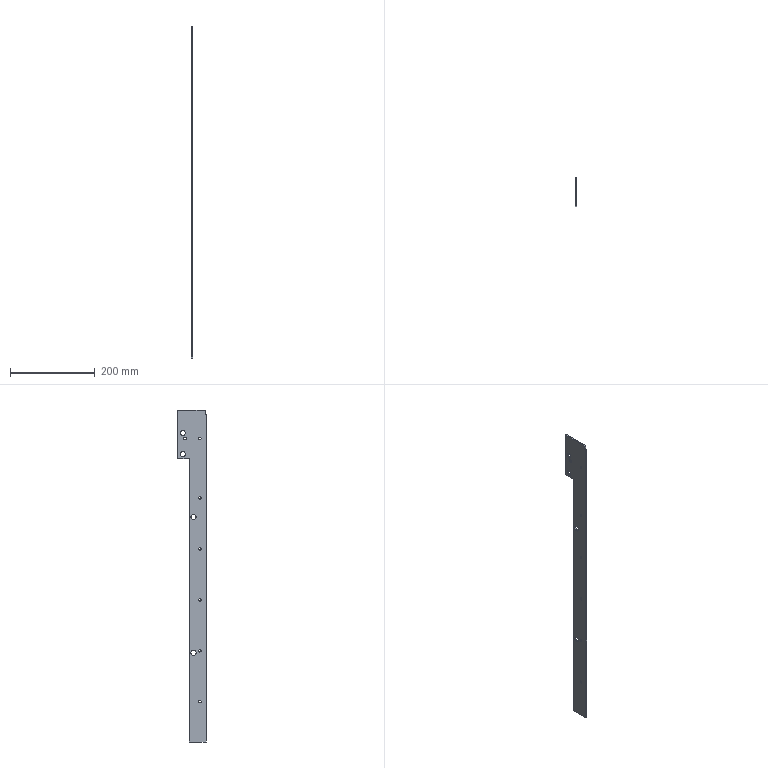Part | NX | features solid 2 | 1 solid | 32 faces | box 3 x 67 x 782.061 mm | volume 101080 mm3 | cylinder 22 | plane 10 | commonest cylinder face diameters 6 x14 12 x8
STEP:
#1=CARTESIAN_POINT('',(1112.,-680.,505.));
#2=VERTEX_POINT('',#1);
#3=CARTESIAN_POINT('',(1112.,-720.,505.));
#4=VERTEX_POINT('',#3);
#5=CARTESIAN_POINT('',(1112.,-1653.,505.));
#6=DIRECTION('',(0.,-1.,0.));
#7=VECTOR('',#6,1000.);
#8=LINE('',#5,#7);
#9=EDGE_CURVE('',#2,#4,#8,.T.);
#10=ORIENTED_EDGE('',*,*,#9,.F.);
#11=CARTESIAN_POINT('',(1115.,-680.,505.));
#12=VERTEX_POINT('',#11);
#13=CARTESIAN_POINT('',(1115.,-680.,505.));
#14=DIRECTION('',(1.,0.,0.));
#15=VECTOR('',#14,1000.);
#16=LINE('',#13,#15);
#17=EDGE_CURVE('',#2,#12,#16,.T.);
#18=ORIENTED_EDGE('',*,*,#17,.T.);
#19=CARTESIAN_POINT('',(1115.,-720.,505.));
#20=VERTEX_POINT('',#19);
#21=CARTESIAN_POINT('',(1115.,-1653.,505.));
#22=DIRECTION('',(0.,-1.,0.));
#23=VECTOR('',#22,1000.);
#24=LINE('',#21,#23);
#25=EDGE_CURVE('',#12,#20,#24,.T.);
#26=ORIENTED_EDGE('',*,*,#25,.T.);
#27=CARTESIAN_POINT('',(1115.,-720.,505.));
#28=DIRECTION('',(1.,0.,0.));
#29=VECTOR('',#28,1000.);
#30=LINE('',#27,#29);
#31=EDGE_CURVE('',#4,#20,#30,.T.);
#32=ORIENTED_EDGE('',*,*,#31,.F.);
#33=EDGE_LOOP('',(#10,#18,#26,#32));
#34=FACE_BOUND('',#33,.T.);
#35=CARTESIAN_POINT('',(1115.,-1653.,505.));
#36=DIRECTION('',(0.,0.,-1.));
#37=DIRECTION('',(0.,-1.,0.));
#38=AXIS2_PLACEMENT_3D('',#35,#36,#37);
#39=PLANE('',#38);
#40=ADVANCED_FACE('',(#34),#39,.T.);
#41=CARTESIAN_POINT('',(1112.,-717.38,1276.152));
#42=VERTEX_POINT('',#41);
#43=CARTESIAN_POINT('',(1112.,-717.38,1287.061));
#44=VERTEX_POINT('',#43);
#45=CARTESIAN_POINT('',(1112.,-717.38,0.));
#46=DIRECTION('',(0.,0.,1.));
#47=VECTOR('',#46,1000.);
#48=LINE('',#45,#47);
#49=EDGE_CURVE('',#42,#44,#48,.T.);
#50=ORIENTED_EDGE('',*,*,#49,.F.);
#51=CARTESIAN_POINT('',(1115.,-717.38,1276.152));
#52=VERTEX_POINT('',#51);
#53=CARTESIAN_POINT('',(1115.,-717.38,1276.152));
#54=DIRECTION('',(1.,0.,0.));
#55=VECTOR('',#54,1000.);
#56=LINE('',#53,#55);
#57=EDGE_CURVE('',#42,#52,#56,.T.);
#58=ORIENTED_EDGE('',*,*,#57,.T.);
#59=CARTESIAN_POINT('',(1115.,-717.38,1287.061));
#60=VERTEX_POINT('',#59);
#61=CARTESIAN_POINT('',(1115.,-717.38,0.));
#62=DIRECTION('',(0.,0.,1.));
#63=VECTOR('',#62,1000.);
#64=LINE('',#61,#63);
#65=EDGE_CURVE('',#52,#60,#64,.T.);
#66=ORIENTED_EDGE('',*,*,#65,.T.);
#67=CARTESIAN_POINT('',(1115.,-717.38,1287.061));
#68=DIRECTION('',(1.,0.,0.));
#69=VECTOR('',#68,1000.);
#70=LINE('',#67,#69);
#71=EDGE_CURVE('',#44,#60,#70,.T.);
#72=ORIENTED_EDGE('',*,*,#71,.F.);
#73=EDGE_LOOP('',(#50,#58,#66,#72));
#74=FACE_BOUND('',#73,.T.);
#75=CARTESIAN_POINT('',(1115.,-717.38,0.));
#76=DIRECTION('',(0.,-1.,0.));
#77=DIRECTION('',(-1.,0.,0.));
#78=AXIS2_PLACEMENT_3D('',#75,#76,#77);
#79=PLANE('',#78);
#80=ADVANCED_FACE('',(#74),#79,.T.);
#81=CARTESIAN_POINT('',(1112.,-720.,1276.152));
#82=VERTEX_POINT('',#81);
#83=CARTESIAN_POINT('',(1115.,-720.,1276.152));
#84=VERTEX_POINT('',#83);
#85=CARTESIAN_POINT('',(1115.,-720.,1276.152));
#86=DIRECTION('',(1.,0.,0.));
#87=VECTOR('',#86,1000.);
#88=LINE('',#85,#87);
#89=EDGE_CURVE('',#82,#84,#88,.T.);
#90=ORIENTED_EDGE('',*,*,#89,.T.);
#91=CARTESIAN_POINT('',(1115.,-1653.,1276.152));
#92=DIRECTION('',(0.,1.,0.));
#93=VECTOR('',#92,1000.);
#94=LINE('',#91,#93);
#95=EDGE_CURVE('',#84,#52,#94,.T.);
#96=ORIENTED_EDGE('',*,*,#95,.T.);
#97=ORIENTED_EDGE('',*,*,#57,.F.);
#98=CARTESIAN_POINT('',(1112.,-1653.,1276.152));
#99=DIRECTION('',(0.,1.,0.));
#100=VECTOR('',#99,1000.);
#101=LINE('',#98,#100);
#102=EDGE_CURVE('',#82,#42,#101,.T.);
#103=ORIENTED_EDGE('',*,*,#102,.F.);
#104=EDGE_LOOP('',(#90,#96,#97,#103));
#105=FACE_BOUND('',#104,.T.);
#106=CARTESIAN_POINT('',(1115.,-1653.,1276.152));
#107=DIRECTION('',(0.,0.,1.));
#108=DIRECTION('',(0.,-1.,0.));
#109=AXIS2_PLACEMENT_3D('',#106,#107,#108);
#110=PLANE('',#109);
#111=ADVANCED_FACE('',(#105),#110,.T.);
#112=CARTESIAN_POINT('',(1112.,-653.,1172.63));
#113=VERTEX_POINT('',#112);
#114=CARTESIAN_POINT('',(1115.,-653.,1172.63));
#115=VERTEX_POINT('',#114);
#116=CARTESIAN_POINT('',(1115.,-653.,1172.63));
#117=DIRECTION('',(1.,0.,0.));
#118=VECTOR('',#117,1000.);
#119=LINE('',#116,#118);
#120=EDGE_CURVE('',#113,#115,#119,.T.);
#121=ORIENTED_EDGE('',*,*,#120,.T.);
#122=CARTESIAN_POINT('',(1115.,-680.,1172.63));
#123=VERTEX_POINT('',#122);
#124=CARTESIAN_POINT('',(1115.,-1653.,1172.63));
#125=DIRECTION('',(0.,-1.,0.));
#126=VECTOR('',#125,1000.);
#127=LINE('',#124,#126);
#128=EDGE_CURVE('',#115,#123,#127,.T.);
#129=ORIENTED_EDGE('',*,*,#128,.T.);
#130=CARTESIAN_POINT('',(1112.,-680.,1172.63));
#131=VERTEX_POINT('',#130);
#132=CARTESIAN_POINT('',(1115.,-680.,1172.63));
#133=DIRECTION('',(1.,0.,0.));
#134=VECTOR('',#133,1000.);
#135=LINE('',#132,#134);
#136=EDGE_CURVE('',#131,#123,#135,.T.);
#137=ORIENTED_EDGE('',*,*,#136,.F.);
#138=CARTESIAN_POINT('',(1112.,-1653.,1172.63));
#139=DIRECTION('',(0.,1.,0.));
#140=VECTOR('',#139,1000.);
#141=LINE('',#138,#140);
#142=EDGE_CURVE('',#131,#113,#141,.T.);
#143=ORIENTED_EDGE('',*,*,#142,.T.);
#144=EDGE_LOOP('',(#121,#129,#137,#143));
#145=FACE_BOUND('',#144,.T.);
#146=CARTESIAN_POINT('',(1115.,-1653.,1172.63));
#147=DIRECTION('',(0.,0.,-1.));
#148=DIRECTION('',(0.,-1.,0.));
#149=AXIS2_PLACEMENT_3D('',#146,#147,#148);
#150=PLANE('',#149);
#151=ADVANCED_FACE('',(#145),#150,.T.);
#152=CARTESIAN_POINT('',(1115.,-680.,0.));
#153=DIRECTION('',(0.,0.,1.));
#154=VECTOR('',#153,1000.);
#155=LINE('',#152,#154);
#156=EDGE_CURVE('',#12,#123,#155,.T.);
#157=ORIENTED_EDGE('',*,*,#156,.F.);
#158=ORIENTED_EDGE('',*,*,#17,.F.);
#159=CARTESIAN_POINT('',(1112.,-680.,0.));
#160=DIRECTION('',(0.,0.,1.));
#161=VECTOR('',#160,1000.);
#162=LINE('',#159,#161);
#163=EDGE_CURVE('',#2,#131,#162,.T.);
#164=ORIENTED_EDGE('',*,*,#163,.T.);
#165=ORIENTED_EDGE('',*,*,#136,.T.);
#166=EDGE_LOOP('',(#157,#158,#164,#165));
#167=FACE_BOUND('',#166,.T.);
#168=CARTESIAN_POINT('',(1115.,-680.,0.));
#169=DIRECTION('',(0.,-1.,0.));
#170=DIRECTION('',(-1.,0.,0.));
#171=AXIS2_PLACEMENT_3D('',#168,#169,#170);
#172=PLANE('',#171);
#173=ADVANCED_FACE('',(#167),#172,.F.);
#174=CARTESIAN_POINT('',(1112.,-690.,709.));
#175=VERTEX_POINT('',#174);
#176=CARTESIAN_POINT('',(1115.,-690.,709.));
#177=VERTEX_POINT('',#176);
#178=CARTESIAN_POINT('',(-391.665,-690.,709.));
#179=DIRECTION('',(1.,0.,0.));
#180=VECTOR('',#179,1000.);
#181=LINE('',#178,#180);
#182=EDGE_CURVE('',#175,#177,#181,.T.);
#183=ORIENTED_EDGE('',*,*,#182,.F.);
#184=CARTESIAN_POINT('',(1112.,-690.,721.));
#185=VERTEX_POINT('',#184);
#186=CARTESIAN_POINT('',(1112.,-690.,715.));
#187=DIRECTION('',(-1.,0.,0.));
#188=DIRECTION('',(0.,0.,-1.));
#189=AXIS2_PLACEMENT_3D('',#186,#187,#188);
#190=CIRCLE('',#189,6.);
#191=EDGE_CURVE('',#175,#185,#190,.T.);
#192=ORIENTED_EDGE('',*,*,#191,.T.);
#193=CARTESIAN_POINT('',(1115.,-690.,721.));
#194=VERTEX_POINT('',#193);
#195=CARTESIAN_POINT('',(-391.665,-690.,721.));
#196=DIRECTION('',(1.,0.,0.));
#197=VECTOR('',#196,1000.);
#198=LINE('',#195,#197);
#199=EDGE_CURVE('',#194,#185,#198,.F.);
#200=ORIENTED_EDGE('',*,*,#199,.F.);
#201=CARTESIAN_POINT('',(1115.,-690.,715.));
#202=DIRECTION('',(1.,0.,0.));
#203=DIRECTION('',(0.,0.,-1.));
#204=AXIS2_PLACEMENT_3D('',#201,#202,#203);
#205=CIRCLE('',#204,6.);
#206=EDGE_CURVE('',#194,#177,#205,.T.);
#207=ORIENTED_EDGE('',*,*,#206,.T.);
#208=EDGE_LOOP('',(#183,#192,#200,#207));
#209=FACE_BOUND('',#208,.T.);
#210=CARTESIAN_POINT('',(-391.665,-690.,715.));
#211=DIRECTION('',(1.,0.,0.));
#212=DIRECTION('',(0.,0.,1.));
#213=AXIS2_PLACEMENT_3D('',#210,#211,#212);
#214=CYLINDRICAL_SURFACE('',#213,6.);
#215=ADVANCED_FACE('',(#209),#214,.F.);
#216=CARTESIAN_POINT('',(1115.,-690.,1029.));
#217=VERTEX_POINT('',#216);
#218=CARTESIAN_POINT('',(1112.,-690.,1029.));
#219=VERTEX_POINT('',#218);
#220=CARTESIAN_POINT('',(-391.665,-690.,1029.));
#221=DIRECTION('',(1.,0.,0.));
#222=VECTOR('',#221,1000.);
#223=LINE('',#220,#222);
#224=EDGE_CURVE('',#217,#219,#223,.F.);
#225=ORIENTED_EDGE('',*,*,#224,.T.);
#226=CARTESIAN_POINT('',(1112.,-690.,1041.));
#227=VERTEX_POINT('',#226);
#228=CARTESIAN_POINT('',(1112.,-690.,1035.));
#229=DIRECTION('',(-1.,0.,0.));
#230=DIRECTION('',(0.,0.,-1.));
#231=AXIS2_PLACEMENT_3D('',#228,#229,#230);
#232=CIRCLE('',#231,6.);
#233=EDGE_CURVE('',#219,#227,#232,.T.);
#234=ORIENTED_EDGE('',*,*,#233,.T.);
#235=CARTESIAN_POINT('',(1115.,-690.,1041.));
#236=VERTEX_POINT('',#235);
#237=CARTESIAN_POINT('',(-391.665,-690.,1041.));
#238=DIRECTION('',(1.,0.,0.));
#239=VECTOR('',#238,1000.);
#240=LINE('',#237,#239);
#241=EDGE_CURVE('',#227,#236,#240,.T.);
#242=ORIENTED_EDGE('',*,*,#241,.T.);
#243=CARTESIAN_POINT('',(1115.,-690.,1035.));
#244=DIRECTION('',(1.,0.,0.));
#245=DIRECTION('',(0.,0.,-1.));
#246=AXIS2_PLACEMENT_3D('',#243,#244,#245);
#247=CIRCLE('',#246,6.);
#248=EDGE_CURVE('',#236,#217,#247,.T.);
#249=ORIENTED_EDGE('',*,*,#248,.T.);
#250=EDGE_LOOP('',(#225,#234,#242,#249));
#251=FACE_BOUND('',#250,.T.);
#252=CARTESIAN_POINT('',(-391.665,-690.,1035.));
#253=DIRECTION('',(1.,0.,0.));
#254=DIRECTION('',(0.,0.,1.));
#255=AXIS2_PLACEMENT_3D('',#252,#253,#254);
#256=CYLINDRICAL_SURFACE('',#255,6.);
#257=ADVANCED_FACE('',(#251),#256,.F.);
#258=CARTESIAN_POINT('',(1112.,-665.,1177.061));
#259=VERTEX_POINT('',#258);
#260=CARTESIAN_POINT('',(1115.,-665.,1177.061));
#261=VERTEX_POINT('',#260);
#262=CARTESIAN_POINT('',(-391.665,-665.,1177.061));
#263=DIRECTION('',(1.,0.,0.));
#264=VECTOR('',#263,1000.);
#265=LINE('',#262,#264);
#266=EDGE_CURVE('',#259,#261,#265,.T.);
#267=ORIENTED_EDGE('',*,*,#266,.F.);
#268=CARTESIAN_POINT('',(1112.,-665.,1189.061));
#269=VERTEX_POINT('',#268);
#270=CARTESIAN_POINT('',(1112.,-665.,1183.061));
#271=DIRECTION('',(-1.,0.,0.));
#272=DIRECTION('',(0.,0.,-1.));
#273=AXIS2_PLACEMENT_3D('',#270,#271,#272);
#274=CIRCLE('',#273,6.);
#275=EDGE_CURVE('',#259,#269,#274,.T.);
#276=ORIENTED_EDGE('',*,*,#275,.T.);
#277=CARTESIAN_POINT('',(1115.,-665.,1189.061));
#278=VERTEX_POINT('',#277);
#279=CARTESIAN_POINT('',(-391.665,-665.,1189.061));
#280=DIRECTION('',(1.,0.,0.));
#281=VECTOR('',#280,1000.);
#282=LINE('',#279,#281);
#283=EDGE_CURVE('',#278,#269,#282,.F.);
#284=ORIENTED_EDGE('',*,*,#283,.F.);
#285=CARTESIAN_POINT('',(1115.,-665.,1183.061));
#286=DIRECTION('',(1.,0.,0.));
#287=DIRECTION('',(0.,0.,-1.));
#288=AXIS2_PLACEMENT_3D('',#285,#286,#287);
#289=CIRCLE('',#288,6.);
#290=EDGE_CURVE('',#278,#261,#289,.T.);
#291=ORIENTED_EDGE('',*,*,#290,.T.);
#292=EDGE_LOOP('',(#267,#276,#284,#291));
#293=FACE_BOUND('',#292,.T.);
#294=CARTESIAN_POINT('',(-391.665,-665.,1183.061));
#295=DIRECTION('',(1.,0.,0.));
#296=DIRECTION('',(0.,0.,1.));
#297=AXIS2_PLACEMENT_3D('',#294,#295,#296);
#298=CYLINDRICAL_SURFACE('',#297,6.);
#299=ADVANCED_FACE('',(#293),#298,.F.);
#300=CARTESIAN_POINT('',(1115.,-665.,1227.061));
#301=VERTEX_POINT('',#300);
#302=CARTESIAN_POINT('',(1112.,-665.,1227.061));
#303=VERTEX_POINT('',#302);
#304=CARTESIAN_POINT('',(-391.665,-665.,1227.061));
#305=DIRECTION('',(1.,0.,0.));
#306=VECTOR('',#305,1000.);
#307=LINE('',#304,#306);
#308=EDGE_CURVE('',#301,#303,#307,.F.);
#309=ORIENTED_EDGE('',*,*,#308,.T.);
#310=CARTESIAN_POINT('',(1112.,-665.,1239.061));
#311=VERTEX_POINT('',#310);
#312=CARTESIAN_POINT('',(1112.,-665.,1233.061));
#313=DIRECTION('',(-1.,0.,0.));
#314=DIRECTION('',(0.,0.,-1.));
#315=AXIS2_PLACEMENT_3D('',#312,#313,#314);
#316=CIRCLE('',#315,6.);
#317=EDGE_CURVE('',#303,#311,#316,.T.);
#318=ORIENTED_EDGE('',*,*,#317,.T.);
#319=CARTESIAN_POINT('',(1115.,-665.,1239.061));
#320=VERTEX_POINT('',#319);
#321=CARTESIAN_POINT('',(-391.665,-665.,1239.061));
#322=DIRECTION('',(1.,0.,0.));
#323=VECTOR('',#322,1000.);
#324=LINE('',#321,#323);
#325=EDGE_CURVE('',#311,#320,#324,.T.);
#326=ORIENTED_EDGE('',*,*,#325,.T.);
#327=CARTESIAN_POINT('',(1115.,-665.,1233.061));
#328=DIRECTION('',(1.,0.,0.));
#329=DIRECTION('',(0.,0.,-1.));
#330=AXIS2_PLACEMENT_3D('',#327,#328,#329);
#331=CIRCLE('',#330,6.);
#332=EDGE_CURVE('',#320,#301,#331,.T.);
#333=ORIENTED_EDGE('',*,*,#332,.T.);
#334=EDGE_LOOP('',(#309,#318,#326,#333));
#335=FACE_BOUND('',#334,.T.);
#336=CARTESIAN_POINT('',(-391.665,-665.,1233.061));
#337=DIRECTION('',(1.,0.,0.));
#338=DIRECTION('',(0.,0.,1.));
#339=AXIS2_PLACEMENT_3D('',#336,#337,#338);
#340=CYLINDRICAL_SURFACE('',#339,6.);
#341=ADVANCED_FACE('',(#335),#340,.F.);
#342=CARTESIAN_POINT('',(1112.,-705.,1217.));
#343=VERTEX_POINT('',#342);
#344=CARTESIAN_POINT('',(1115.,-705.,1217.));
#345=VERTEX_POINT('',#344);
#346=CARTESIAN_POINT('',(-391.665,-705.,1217.));
#347=DIRECTION('',(1.,0.,0.));
#348=VECTOR('',#347,1000.);
#349=LINE('',#346,#348);
#350=EDGE_CURVE('',#343,#345,#349,.T.);
#351=ORIENTED_EDGE('',*,*,#350,.F.);
#352=CARTESIAN_POINT('',(1112.,-705.,1223.));
#353=VERTEX_POINT('',#352);
#354=CARTESIAN_POINT('',(1112.,-705.,1220.));
#355=DIRECTION('',(1.,0.,0.));
#356=DIRECTION('',(0.,0.,-1.));
#357=AXIS2_PLACEMENT_3D('',#354,#355,#356);
#358=CIRCLE('',#357,3.);
#359=EDGE_CURVE('',#353,#343,#358,.T.);
#360=ORIENTED_EDGE('',*,*,#359,.F.);
#361=CARTESIAN_POINT('',(1115.,-705.,1223.));
#362=VERTEX_POINT('',#361);
#363=CARTESIAN_POINT('',(-391.665,-705.,1223.));
#364=DIRECTION('',(1.,0.,0.));
#365=VECTOR('',#364,1000.);
#366=LINE('',#363,#365);
#367=EDGE_CURVE('',#362,#353,#366,.F.);
#368=ORIENTED_EDGE('',*,*,#367,.F.);
#369=CARTESIAN_POINT('',(1115.,-705.,1220.));
#370=DIRECTION('',(-1.,0.,0.));
#371=DIRECTION('',(0.,1.,0.));
#372=AXIS2_PLACEMENT_3D('',#369,#370,#371);
#373=CIRCLE('',#372,3.);
#374=EDGE_CURVE('',#345,#362,#373,.T.);
#375=ORIENTED_EDGE('',*,*,#374,.F.);
#376=EDGE_LOOP('',(#351,#360,#368,#375));
#377=FACE_BOUND('',#376,.T.);
#378=CARTESIAN_POINT('',(-391.665,-705.,1220.));
#379=DIRECTION('',(1.,0.,0.));
#380=DIRECTION('',(0.,0.,1.));
#381=AXIS2_PLACEMENT_3D('',#378,#379,#380);
#382=CYLINDRICAL_SURFACE('',#381,3.);
#383=ADVANCED_FACE('',(#377),#382,.F.);
#384=CARTESIAN_POINT('',(1112.,-670.,1217.));
#385=VERTEX_POINT('',#384);
#386=CARTESIAN_POINT('',(1115.,-670.,1217.));
#387=VERTEX_POINT('',#386);
#388=CARTESIAN_POINT('',(-391.665,-670.,1217.));
#389=DIRECTION('',(1.,0.,0.));
#390=VECTOR('',#389,1000.);
#391=LINE('',#388,#390);
#392=EDGE_CURVE('',#385,#387,#391,.T.);
#393=ORIENTED_EDGE('',*,*,#392,.F.);
#394=CARTESIAN_POINT('',(1112.,-670.,1223.));
#395=VERTEX_POINT('',#394);
#396=CARTESIAN_POINT('',(1112.,-670.,1220.));
#397=DIRECTION('',(1.,0.,0.));
#398=DIRECTION('',(0.,0.,-1.));
#399=AXIS2_PLACEMENT_3D('',#396,#397,#398);
#400=CIRCLE('',#399,3.);
#401=EDGE_CURVE('',#395,#385,#400,.T.);
#402=ORIENTED_EDGE('',*,*,#401,.F.);
#403=CARTESIAN_POINT('',(1115.,-670.,1223.));
#404=VERTEX_POINT('',#403);
#405=CARTESIAN_POINT('',(-391.665,-670.,1223.));
#406=DIRECTION('',(1.,0.,0.));
#407=VECTOR('',#406,1000.);
#408=LINE('',#405,#407);
#409=EDGE_CURVE('',#404,#395,#408,.F.);
#410=ORIENTED_EDGE('',*,*,#409,.F.);
#411=CARTESIAN_POINT('',(1115.,-670.,1220.));
#412=DIRECTION('',(-1.,0.,0.));
#413=DIRECTION('',(0.,1.,0.));
#414=AXIS2_PLACEMENT_3D('',#411,#412,#413);
#415=CIRCLE('',#414,3.);
#416=EDGE_CURVE('',#387,#404,#415,.T.);
#417=ORIENTED_EDGE('',*,*,#416,.F.);
#418=EDGE_LOOP('',(#393,#402,#410,#417));
#419=FACE_BOUND('',#418,.T.);
#420=CARTESIAN_POINT('',(-391.665,-670.,1220.));
#421=DIRECTION('',(1.,0.,0.));
#422=DIRECTION('',(0.,0.,1.));
#423=AXIS2_PLACEMENT_3D('',#420,#421,#422);
#424=CYLINDRICAL_SURFACE('',#423,3.);
#425=ADVANCED_FACE('',(#419),#424,.F.);
#426=CARTESIAN_POINT('',(1115.,-705.,1077.));
#427=VERTEX_POINT('',#426);
#428=CARTESIAN_POINT('',(1112.,-705.,1077.));
#429=VERTEX_POINT('',#428);
#430=CARTESIAN_POINT('',(-391.665,-705.,1077.));
#431=DIRECTION('',(1.,0.,0.));
#432=VECTOR('',#431,1000.);
#433=LINE('',#430,#432);
#434=EDGE_CURVE('',#427,#429,#433,.F.);
#435=ORIENTED_EDGE('',*,*,#434,.T.);
#436=CARTESIAN_POINT('',(1112.,-705.,1083.));
#437=VERTEX_POINT('',#436);
#438=CARTESIAN_POINT('',(1112.,-705.,1080.));
#439=DIRECTION('',(1.,0.,0.));
#440=DIRECTION('',(0.,0.,-1.));
#441=AXIS2_PLACEMENT_3D('',#438,#439,#440);
#442=CIRCLE('',#441,3.);
#443=EDGE_CURVE('',#437,#429,#442,.T.);
#444=ORIENTED_EDGE('',*,*,#443,.F.);
#445=CARTESIAN_POINT('',(1115.,-705.,1083.));
#446=VERTEX_POINT('',#445);
#447=CARTESIAN_POINT('',(-391.665,-705.,1083.));
#448=DIRECTION('',(1.,0.,0.));
#449=VECTOR('',#448,1000.);
#450=LINE('',#447,#449);
#451=EDGE_CURVE('',#437,#446,#450,.T.);
#452=ORIENTED_EDGE('',*,*,#451,.T.);
#453=CARTESIAN_POINT('',(1115.,-705.,1080.));
#454=DIRECTION('',(-1.,0.,0.));
#455=DIRECTION('',(0.,1.,0.));
#456=AXIS2_PLACEMENT_3D('',#453,#454,#455);
#457=CIRCLE('',#456,3.);
#458=EDGE_CURVE('',#427,#446,#457,.T.);
#459=ORIENTED_EDGE('',*,*,#458,.F.);
#460=EDGE_LOOP('',(#435,#444,#452,#459));
#461=FACE_BOUND('',#460,.T.);
#462=CARTESIAN_POINT('',(-391.665,-705.,1080.));
#463=DIRECTION('',(1.,0.,0.));
#464=DIRECTION('',(0.,0.,1.));
#465=AXIS2_PLACEMENT_3D('',#462,#463,#464);
#466=CYLINDRICAL_SURFACE('',#465,3.);
#467=ADVANCED_FACE('',(#461),#466,.F.);
#468=CARTESIAN_POINT('',(1112.,-705.,957.));
#469=VERTEX_POINT('',#468);
#470=CARTESIAN_POINT('',(1115.,-705.,957.));
#471=VERTEX_POINT('',#470);
#472=CARTESIAN_POINT('',(-391.665,-705.,957.));
#473=DIRECTION('',(1.,0.,0.));
#474=VECTOR('',#473,1000.);
#475=LINE('',#472,#474);
#476=EDGE_CURVE('',#469,#471,#475,.T.);
#477=ORIENTED_EDGE('',*,*,#476,.F.);
#478=CARTESIAN_POINT('',(1112.,-705.,963.));
#479=VERTEX_POINT('',#478);
#480=CARTESIAN_POINT('',(1112.,-705.,960.));
#481=DIRECTION('',(1.,0.,0.));
#482=DIRECTION('',(0.,0.,-1.));
#483=AXIS2_PLACEMENT_3D('',#480,#481,#482);
#484=CIRCLE('',#483,3.);
#485=EDGE_CURVE('',#479,#469,#484,.T.);
#486=ORIENTED_EDGE('',*,*,#485,.F.);
#487=CARTESIAN_POINT('',(1115.,-705.,963.));
#488=VERTEX_POINT('',#487);
#489=CARTESIAN_POINT('',(-391.665,-705.,963.));
#490=DIRECTION('',(1.,0.,0.));
#491=VECTOR('',#490,1000.);
#492=LINE('',#489,#491);
#493=EDGE_CURVE('',#488,#479,#492,.F.);
#494=ORIENTED_EDGE('',*,*,#493,.F.);
#495=CARTESIAN_POINT('',(1115.,-705.,960.));
#496=DIRECTION('',(-1.,0.,0.));
#497=DIRECTION('',(0.,1.,0.));
#498=AXIS2_PLACEMENT_3D('',#495,#496,#497);
#499=CIRCLE('',#498,3.);
#500=EDGE_CURVE('',#471,#488,#499,.T.);
#501=ORIENTED_EDGE('',*,*,#500,.F.);
#502=EDGE_LOOP('',(#477,#486,#494,#501));
#503=FACE_BOUND('',#502,.T.);
#504=CARTESIAN_POINT('',(-391.665,-705.,960.));
#505=DIRECTION('',(1.,0.,0.));
#506=DIRECTION('',(0.,0.,1.));
#507=AXIS2_PLACEMENT_3D('',#504,#505,#506);
#508=CYLINDRICAL_SURFACE('',#507,3.);
#509=ADVANCED_FACE('',(#503),#508,.F.);
#510=CARTESIAN_POINT('',(1115.,-705.,837.));
#511=VERTEX_POINT('',#510);
#512=CARTESIAN_POINT('',(1112.,-705.,837.));
#513=VERTEX_POINT('',#512);
#514=CARTESIAN_POINT('',(-391.665,-705.,837.));
#515=DIRECTION('',(1.,0.,0.));
#516=VECTOR('',#515,1000.);
#517=LINE('',#514,#516);
#518=EDGE_CURVE('',#511,#513,#517,.F.);
#519=ORIENTED_EDGE('',*,*,#518,.T.);
#520=CARTESIAN_POINT('',(1112.,-705.,843.));
#521=VERTEX_POINT('',#520);
#522=CARTESIAN_POINT('',(1112.,-705.,840.));
#523=DIRECTION('',(1.,0.,0.));
#524=DIRECTION('',(0.,0.,-1.));
#525=AXIS2_PLACEMENT_3D('',#522,#523,#524);
#526=CIRCLE('',#525,3.);
#527=EDGE_CURVE('',#521,#513,#526,.T.);
#528=ORIENTED_EDGE('',*,*,#527,.F.);
#529=CARTESIAN_POINT('',(1115.,-705.,843.));
#530=VERTEX_POINT('',#529);
#531=CARTESIAN_POINT('',(-391.665,-705.,843.));
#532=DIRECTION('',(1.,0.,0.));
#533=VECTOR('',#532,1000.);
#534=LINE('',#531,#533);
#535=EDGE_CURVE('',#521,#530,#534,.T.);
#536=ORIENTED_EDGE('',*,*,#535,.T.);
#537=CARTESIAN_POINT('',(1115.,-705.,840.));
#538=DIRECTION('',(-1.,0.,0.));
#539=DIRECTION('',(0.,1.,0.));
#540=AXIS2_PLACEMENT_3D('',#537,#538,#539);
#541=CIRCLE('',#540,3.);
#542=EDGE_CURVE('',#511,#530,#541,.T.);
#543=ORIENTED_EDGE('',*,*,#542,.F.);
#544=EDGE_LOOP('',(#519,#528,#536,#543));
#545=FACE_BOUND('',#544,.T.);
#546=CARTESIAN_POINT('',(-391.665,-705.,840.));
#547=DIRECTION('',(1.,0.,0.));
#548=DIRECTION('',(0.,0.,1.));
#549=AXIS2_PLACEMENT_3D('',#546,#547,#548);
#550=CYLINDRICAL_SURFACE('',#549,3.);
#551=ADVANCED_FACE('',(#545),#550,.F.);
#552=CARTESIAN_POINT('',(1112.,-705.,717.));
#553=VERTEX_POINT('',#552);
#554=CARTESIAN_POINT('',(1115.,-705.,717.));
#555=VERTEX_POINT('',#554);
#556=CARTESIAN_POINT('',(-391.665,-705.,717.));
#557=DIRECTION('',(1.,0.,0.));
#558=VECTOR('',#557,1000.);
#559=LINE('',#556,#558);
#560=EDGE_CURVE('',#553,#555,#559,.T.);
#561=ORIENTED_EDGE('',*,*,#560,.F.);
#562=CARTESIAN_POINT('',(1112.,-705.,723.));
#563=VERTEX_POINT('',#562);
#564=CARTESIAN_POINT('',(1112.,-705.,720.));
#565=DIRECTION('',(1.,0.,0.));
#566=DIRECTION('',(0.,0.,-1.));
#567=AXIS2_PLACEMENT_3D('',#564,#565,#566);
#568=CIRCLE('',#567,3.);
#569=EDGE_CURVE('',#563,#553,#568,.T.);
#570=ORIENTED_EDGE('',*,*,#569,.F.);
#571=CARTESIAN_POINT('',(1115.,-705.,723.));
#572=VERTEX_POINT('',#571);
#573=CARTESIAN_POINT('',(-391.665,-705.,723.));
#574=DIRECTION('',(1.,0.,0.));
#575=VECTOR('',#574,1000.);
#576=LINE('',#573,#575);
#577=EDGE_CURVE('',#572,#563,#576,.F.);
#578=ORIENTED_EDGE('',*,*,#577,.F.);
#579=CARTESIAN_POINT('',(1115.,-705.,720.));
#580=DIRECTION('',(-1.,0.,0.));
#581=DIRECTION('',(0.,1.,0.));
#582=AXIS2_PLACEMENT_3D('',#579,#580,#581);
#583=CIRCLE('',#582,3.);
#584=EDGE_CURVE('',#555,#572,#583,.T.);
#585=ORIENTED_EDGE('',*,*,#584,.F.);
#586=EDGE_LOOP('',(#561,#570,#578,#585));
#587=FACE_BOUND('',#586,.T.);
#588=CARTESIAN_POINT('',(-391.665,-705.,720.));
#589=DIRECTION('',(1.,0.,0.));
#590=DIRECTION('',(0.,0.,1.));
#591=AXIS2_PLACEMENT_3D('',#588,#589,#590);
#592=CYLINDRICAL_SURFACE('',#591,3.);
#593=ADVANCED_FACE('',(#587),#592,.F.);
#594=CARTESIAN_POINT('',(1112.,-705.,597.));
#595=VERTEX_POINT('',#594);
#596=CARTESIAN_POINT('',(1115.,-705.,597.));
#597=VERTEX_POINT('',#596);
#598=CARTESIAN_POINT('',(-391.665,-705.,597.));
#599=DIRECTION('',(1.,0.,0.));
#600=VECTOR('',#599,1000.);
#601=LINE('',#598,#600);
#602=EDGE_CURVE('',#595,#597,#601,.T.);
#603=ORIENTED_EDGE('',*,*,#602,.F.);
#604=CARTESIAN_POINT('',(1112.,-705.,603.));
#605=VERTEX_POINT('',#604);
#606=CARTESIAN_POINT('',(1112.,-705.,600.));
#607=DIRECTION('',(1.,0.,0.));
#608=DIRECTION('',(0.,0.,-1.));
#609=AXIS2_PLACEMENT_3D('',#606,#607,#608);
#610=CIRCLE('',#609,3.);
#611=EDGE_CURVE('',#605,#595,#610,.T.);
#612=ORIENTED_EDGE('',*,*,#611,.F.);
#613=CARTESIAN_POINT('',(1115.,-705.,603.));
#614=VERTEX_POINT('',#613);
#615=CARTESIAN_POINT('',(-391.665,-705.,603.));
#616=DIRECTION('',(1.,0.,0.));
#617=VECTOR('',#616,1000.);
#618=LINE('',#615,#617);
#619=EDGE_CURVE('',#614,#605,#618,.F.);
#620=ORIENTED_EDGE('',*,*,#619,.F.);
#621=CARTESIAN_POINT('',(1115.,-705.,600.));
#622=DIRECTION('',(-1.,0.,0.));
#623=DIRECTION('',(0.,1.,0.));
#624=AXIS2_PLACEMENT_3D('',#621,#622,#623);
#625=CIRCLE('',#624,3.);
#626=EDGE_CURVE('',#597,#614,#625,.T.);
#627=ORIENTED_EDGE('',*,*,#626,.F.);
#628=EDGE_LOOP('',(#603,#612,#620,#627));
#629=FACE_BOUND('',#628,.T.);
#630=CARTESIAN_POINT('',(-391.665,-705.,600.));
#631=DIRECTION('',(1.,0.,0.));
#632=DIRECTION('',(0.,0.,1.));
#633=AXIS2_PLACEMENT_3D('',#630,#631,#632);
#634=CYLINDRICAL_SURFACE('',#633,3.);
#635=ADVANCED_FACE('',(#629),#634,.F.);
#636=CARTESIAN_POINT('',(1115.,-705.,600.));
#637=DIRECTION('',(-1.,0.,0.));
#638=DIRECTION('',(0.,1.,0.));
#639=AXIS2_PLACEMENT_3D('',#636,#637,#638);
#640=CIRCLE('',#639,3.);
#641=EDGE_CURVE('',#614,#597,#640,.T.);
#642=ORIENTED_EDGE('',*,*,#641,.T.);
#643=ORIENTED_EDGE('',*,*,#626,.T.);
#644=EDGE_LOOP('',(#642,#643));
#645=FACE_BOUND('',#644,.T.);
#646=CARTESIAN_POINT('',(1115.,-705.,720.));
#647=DIRECTION('',(-1.,0.,0.));
#648=DIRECTION('',(0.,1.,0.));
#649=AXIS2_PLACEMENT_3D('',#646,#647,#648);
#650=CIRCLE('',#649,3.);
#651=EDGE_CURVE('',#572,#555,#650,.T.);
#652=ORIENTED_EDGE('',*,*,#651,.T.);
#653=ORIENTED_EDGE('',*,*,#584,.T.);
#654=EDGE_LOOP('',(#652,#653));
#655=FACE_BOUND('',#654,.T.);
#656=CARTESIAN_POINT('',(1115.,-705.,840.));
#657=DIRECTION('',(-1.,0.,0.));
#658=DIRECTION('',(0.,1.,0.));
#659=AXIS2_PLACEMENT_3D('',#656,#657,#658);
#660=CIRCLE('',#659,3.);
#661=EDGE_CURVE('',#530,#511,#660,.T.);
#662=ORIENTED_EDGE('',*,*,#661,.T.);
#663=ORIENTED_EDGE('',*,*,#542,.T.);
#664=EDGE_LOOP('',(#662,#663));
#665=FACE_BOUND('',#664,.T.);
#666=CARTESIAN_POINT('',(1115.,-705.,960.));
#667=DIRECTION('',(-1.,0.,0.));
#668=DIRECTION('',(0.,1.,0.));
#669=AXIS2_PLACEMENT_3D('',#666,#667,#668);
#670=CIRCLE('',#669,3.);
#671=EDGE_CURVE('',#488,#471,#670,.T.);
#672=ORIENTED_EDGE('',*,*,#671,.T.);
#673=ORIENTED_EDGE('',*,*,#500,.T.);
#674=EDGE_LOOP('',(#672,#673));
#675=FACE_BOUND('',#674,.T.);
#676=CARTESIAN_POINT('',(1115.,-705.,1080.));
#677=DIRECTION('',(-1.,0.,0.));
#678=DIRECTION('',(0.,1.,0.));
#679=AXIS2_PLACEMENT_3D('',#676,#677,#678);
#680=CIRCLE('',#679,3.);
#681=EDGE_CURVE('',#446,#427,#680,.T.);
#682=ORIENTED_EDGE('',*,*,#681,.T.);
#683=ORIENTED_EDGE('',*,*,#458,.T.);
#684=EDGE_LOOP('',(#682,#683));
#685=FACE_BOUND('',#684,.T.);
#686=CARTESIAN_POINT('',(1115.,-670.,1220.));
#687=DIRECTION('',(-1.,0.,0.));
#688=DIRECTION('',(0.,1.,0.));
#689=AXIS2_PLACEMENT_3D('',#686,#687,#688);
#690=CIRCLE('',#689,3.);
#691=EDGE_CURVE('',#404,#387,#690,.T.);
#692=ORIENTED_EDGE('',*,*,#691,.T.);
#693=ORIENTED_EDGE('',*,*,#416,.T.);
#694=EDGE_LOOP('',(#692,#693));
#695=FACE_BOUND('',#694,.T.);
#696=CARTESIAN_POINT('',(1115.,-705.,1220.));
#697=DIRECTION('',(-1.,0.,0.));
#698=DIRECTION('',(0.,1.,0.));
#699=AXIS2_PLACEMENT_3D('',#696,#697,#698);
#700=CIRCLE('',#699,3.);
#701=EDGE_CURVE('',#362,#345,#700,.T.);
#702=ORIENTED_EDGE('',*,*,#701,.T.);
#703=ORIENTED_EDGE('',*,*,#374,.T.);
#704=EDGE_LOOP('',(#702,#703));
#705=FACE_BOUND('',#704,.T.);
#706=ORIENTED_EDGE('',*,*,#332,.F.);
#707=CARTESIAN_POINT('',(1115.,-665.,1233.061));
#708=DIRECTION('',(1.,0.,0.));
#709=DIRECTION('',(0.,0.,-1.));
#710=AXIS2_PLACEMENT_3D('',#707,#708,#709);
#711=CIRCLE('',#710,6.);
#712=EDGE_CURVE('',#301,#320,#711,.T.);
#713=ORIENTED_EDGE('',*,*,#712,.F.);
#714=EDGE_LOOP('',(#706,#713));
#715=FACE_BOUND('',#714,.T.);
#716=ORIENTED_EDGE('',*,*,#290,.F.);
#717=CARTESIAN_POINT('',(1115.,-665.,1183.061));
#718=DIRECTION('',(1.,0.,0.));
#719=DIRECTION('',(0.,0.,-1.));
#720=AXIS2_PLACEMENT_3D('',#717,#718,#719);
#721=CIRCLE('',#720,6.);
#722=EDGE_CURVE('',#261,#278,#721,.T.);
#723=ORIENTED_EDGE('',*,*,#722,.F.);
#724=EDGE_LOOP('',(#716,#723));
#725=FACE_BOUND('',#724,.T.);
#726=ORIENTED_EDGE('',*,*,#248,.F.);
#727=CARTESIAN_POINT('',(1115.,-690.,1035.));
#728=DIRECTION('',(1.,0.,0.));
#729=DIRECTION('',(0.,0.,-1.));
#730=AXIS2_PLACEMENT_3D('',#727,#728,#729);
#731=CIRCLE('',#730,6.);
#732=EDGE_CURVE('',#217,#236,#731,.T.);
#733=ORIENTED_EDGE('',*,*,#732,.F.);
#734=EDGE_LOOP('',(#726,#733));
#735=FACE_BOUND('',#734,.T.);
#736=ORIENTED_EDGE('',*,*,#206,.F.);
#737=CARTESIAN_POINT('',(1115.,-690.,715.));
#738=DIRECTION('',(1.,0.,0.));
#739=DIRECTION('',(0.,0.,-1.));
#740=AXIS2_PLACEMENT_3D('',#737,#738,#739);
#741=CIRCLE('',#740,6.);
#742=EDGE_CURVE('',#177,#194,#741,.T.);
#743=ORIENTED_EDGE('',*,*,#742,.F.);
#744=EDGE_LOOP('',(#736,#743));
#745=FACE_BOUND('',#744,.T.);
#746=CARTESIAN_POINT('',(1115.,-720.,1287.061));
#747=DIRECTION('',(0.,0.,-1.));
#748=VECTOR('',#747,1000.);
#749=LINE('',#746,#748);
#750=EDGE_CURVE('',#84,#20,#749,.T.);
#751=ORIENTED_EDGE('',*,*,#750,.T.);
#752=ORIENTED_EDGE('',*,*,#25,.F.);
#753=ORIENTED_EDGE('',*,*,#156,.T.);
#754=ORIENTED_EDGE('',*,*,#128,.F.);
#755=CARTESIAN_POINT('',(1115.,-653.,1287.061));
#756=VERTEX_POINT('',#755);
#757=CARTESIAN_POINT('',(1115.,-653.,0.));
#758=DIRECTION('',(0.,0.,1.));
#759=VECTOR('',#758,1000.);
#760=LINE('',#757,#759);
#761=EDGE_CURVE('',#115,#756,#760,.T.);
#762=ORIENTED_EDGE('',*,*,#761,.T.);
#763=CARTESIAN_POINT('',(1115.,-720.,1287.061));
#764=DIRECTION('',(0.,-1.,0.));
#765=VECTOR('',#764,1000.);
#766=LINE('',#763,#765);
#767=EDGE_CURVE('',#756,#60,#766,.T.);
#768=ORIENTED_EDGE('',*,*,#767,.T.);
#769=ORIENTED_EDGE('',*,*,#65,.F.);
#770=ORIENTED_EDGE('',*,*,#95,.F.);
#771=EDGE_LOOP('',(#751,#752,#753,#754,#762,#768,#769,#770));
#772=FACE_BOUND('',#771,.T.);
#773=CARTESIAN_POINT('',(1115.,-1653.,0.));
#774=DIRECTION('',(-1.,0.,0.));
#775=DIRECTION('',(0.,0.,1.));
#776=AXIS2_PLACEMENT_3D('',#773,#774,#775);
#777=PLANE('',#776);
#778=ADVANCED_FACE('',(#645,#655,#665,#675,#685,#695,#705,#715,#725,#735,#745,#772),#777,.F.);
#779=ORIENTED_EDGE('',*,*,#611,.T.);
#780=CARTESIAN_POINT('',(1112.,-705.,600.));
#781=DIRECTION('',(1.,0.,0.));
#782=DIRECTION('',(0.,0.,-1.));
#783=AXIS2_PLACEMENT_3D('',#780,#781,#782);
#784=CIRCLE('',#783,3.);
#785=EDGE_CURVE('',#595,#605,#784,.T.);
#786=ORIENTED_EDGE('',*,*,#785,.T.);
#787=EDGE_LOOP('',(#779,#786));
#788=FACE_BOUND('',#787,.T.);
#789=ORIENTED_EDGE('',*,*,#569,.T.);
#790=CARTESIAN_POINT('',(1112.,-705.,720.));
#791=DIRECTION('',(1.,0.,0.));
#792=DIRECTION('',(0.,0.,-1.));
#793=AXIS2_PLACEMENT_3D('',#790,#791,#792);
#794=CIRCLE('',#793,3.);
#795=EDGE_CURVE('',#553,#563,#794,.T.);
#796=ORIENTED_EDGE('',*,*,#795,.T.);
#797=EDGE_LOOP('',(#789,#796));
#798=FACE_BOUND('',#797,.T.);
#799=ORIENTED_EDGE('',*,*,#527,.T.);
#800=CARTESIAN_POINT('',(1112.,-705.,840.));
#801=DIRECTION('',(1.,0.,0.));
#802=DIRECTION('',(0.,0.,-1.));
#803=AXIS2_PLACEMENT_3D('',#800,#801,#802);
#804=CIRCLE('',#803,3.);
#805=EDGE_CURVE('',#513,#521,#804,.T.);
#806=ORIENTED_EDGE('',*,*,#805,.T.);
#807=EDGE_LOOP('',(#799,#806));
#808=FACE_BOUND('',#807,.T.);
#809=ORIENTED_EDGE('',*,*,#485,.T.);
#810=CARTESIAN_POINT('',(1112.,-705.,960.));
#811=DIRECTION('',(1.,0.,0.));
#812=DIRECTION('',(0.,0.,-1.));
#813=AXIS2_PLACEMENT_3D('',#810,#811,#812);
#814=CIRCLE('',#813,3.);
#815=EDGE_CURVE('',#469,#479,#814,.T.);
#816=ORIENTED_EDGE('',*,*,#815,.T.);
#817=EDGE_LOOP('',(#809,#816));
#818=FACE_BOUND('',#817,.T.);
#819=ORIENTED_EDGE('',*,*,#443,.T.);
#820=CARTESIAN_POINT('',(1112.,-705.,1080.));
#821=DIRECTION('',(1.,0.,0.));
#822=DIRECTION('',(0.,0.,-1.));
#823=AXIS2_PLACEMENT_3D('',#820,#821,#822);
#824=CIRCLE('',#823,3.);
#825=EDGE_CURVE('',#429,#437,#824,.T.);
#826=ORIENTED_EDGE('',*,*,#825,.T.);
#827=EDGE_LOOP('',(#819,#826));
#828=FACE_BOUND('',#827,.T.);
#829=ORIENTED_EDGE('',*,*,#401,.T.);
#830=CARTESIAN_POINT('',(1112.,-670.,1220.));
#831=DIRECTION('',(1.,0.,0.));
#832=DIRECTION('',(0.,0.,-1.));
#833=AXIS2_PLACEMENT_3D('',#830,#831,#832);
#834=CIRCLE('',#833,3.);
#835=EDGE_CURVE('',#385,#395,#834,.T.);
#836=ORIENTED_EDGE('',*,*,#835,.T.);
#837=EDGE_LOOP('',(#829,#836));
#838=FACE_BOUND('',#837,.T.);
#839=ORIENTED_EDGE('',*,*,#359,.T.);
#840=CARTESIAN_POINT('',(1112.,-705.,1220.));
#841=DIRECTION('',(1.,0.,0.));
#842=DIRECTION('',(0.,0.,-1.));
#843=AXIS2_PLACEMENT_3D('',#840,#841,#842);
#844=CIRCLE('',#843,3.);
#845=EDGE_CURVE('',#343,#353,#844,.T.);
#846=ORIENTED_EDGE('',*,*,#845,.T.);
#847=EDGE_LOOP('',(#839,#846));
#848=FACE_BOUND('',#847,.T.);
#849=CARTESIAN_POINT('',(1112.,-665.,1233.061));
#850=DIRECTION('',(-1.,0.,0.));
#851=DIRECTION('',(0.,0.,-1.));
#852=AXIS2_PLACEMENT_3D('',#849,#850,#851);
#853=CIRCLE('',#852,6.);
#854=EDGE_CURVE('',#311,#303,#853,.T.);
#855=ORIENTED_EDGE('',*,*,#854,.F.);
#856=ORIENTED_EDGE('',*,*,#317,.F.);
#857=EDGE_LOOP('',(#855,#856));
#858=FACE_BOUND('',#857,.T.);
#859=CARTESIAN_POINT('',(1112.,-665.,1183.061));
#860=DIRECTION('',(-1.,0.,0.));
#861=DIRECTION('',(0.,0.,-1.));
#862=AXIS2_PLACEMENT_3D('',#859,#860,#861);
#863=CIRCLE('',#862,6.);
#864=EDGE_CURVE('',#269,#259,#863,.T.);
#865=ORIENTED_EDGE('',*,*,#864,.F.);
#866=ORIENTED_EDGE('',*,*,#275,.F.);
#867=EDGE_LOOP('',(#865,#866));
#868=FACE_BOUND('',#867,.T.);
#869=CARTESIAN_POINT('',(1112.,-690.,1035.));
#870=DIRECTION('',(-1.,0.,0.));
#871=DIRECTION('',(0.,0.,-1.));
#872=AXIS2_PLACEMENT_3D('',#869,#870,#871);
#873=CIRCLE('',#872,6.);
#874=EDGE_CURVE('',#227,#219,#873,.T.);
#875=ORIENTED_EDGE('',*,*,#874,.F.);
#876=ORIENTED_EDGE('',*,*,#233,.F.);
#877=EDGE_LOOP('',(#875,#876));
#878=FACE_BOUND('',#877,.T.);
#879=CARTESIAN_POINT('',(1112.,-690.,715.));
#880=DIRECTION('',(-1.,0.,0.));
#881=DIRECTION('',(0.,0.,-1.));
#882=AXIS2_PLACEMENT_3D('',#879,#880,#881);
#883=CIRCLE('',#882,6.);
#884=EDGE_CURVE('',#185,#175,#883,.T.);
#885=ORIENTED_EDGE('',*,*,#884,.F.);
#886=ORIENTED_EDGE('',*,*,#191,.F.);
#887=EDGE_LOOP('',(#885,#886));
#888=FACE_BOUND('',#887,.T.);
#889=ORIENTED_EDGE('',*,*,#9,.T.);
#890=CARTESIAN_POINT('',(1112.,-720.,1287.061));
#891=DIRECTION('',(0.,0.,-1.));
#892=VECTOR('',#891,1000.);
#893=LINE('',#890,#892);
#894=EDGE_CURVE('',#82,#4,#893,.T.);
#895=ORIENTED_EDGE('',*,*,#894,.F.);
#896=ORIENTED_EDGE('',*,*,#102,.T.);
#897=ORIENTED_EDGE('',*,*,#49,.T.);
#898=CARTESIAN_POINT('',(1112.,-653.,1287.061));
#899=VERTEX_POINT('',#898);
#900=CARTESIAN_POINT('',(1112.,-720.,1287.061));
#901=DIRECTION('',(0.,-1.,0.));
#902=VECTOR('',#901,1000.);
#903=LINE('',#900,#902);
#904=EDGE_CURVE('',#899,#44,#903,.T.);
#905=ORIENTED_EDGE('',*,*,#904,.F.);
#906=CARTESIAN_POINT('',(1112.,-653.,0.));
#907=DIRECTION('',(0.,0.,1.));
#908=VECTOR('',#907,1000.);
#909=LINE('',#906,#908);
#910=EDGE_CURVE('',#113,#899,#909,.T.);
#911=ORIENTED_EDGE('',*,*,#910,.F.);
#912=ORIENTED_EDGE('',*,*,#142,.F.);
#913=ORIENTED_EDGE('',*,*,#163,.F.);
#914=EDGE_LOOP('',(#889,#895,#896,#897,#905,#911,#912,#913));
#915=FACE_BOUND('',#914,.T.);
#916=CARTESIAN_POINT('',(1112.,-1653.,0.));
#917=DIRECTION('',(-1.,0.,0.));
#918=DIRECTION('',(0.,0.,1.));
#919=AXIS2_PLACEMENT_3D('',#916,#917,#918);
#920=PLANE('',#919);
#921=ADVANCED_FACE('',(#788,#798,#808,#818,#828,#838,#848,#858,#868,#878,#888,#915),#920,.T.);
#922=ORIENTED_EDGE('',*,*,#71,.T.);
#923=ORIENTED_EDGE('',*,*,#767,.F.);
#924=CARTESIAN_POINT('',(1112.,-653.,1287.061));
#925=DIRECTION('',(1.,0.,0.));
#926=VECTOR('',#925,1000.);
#927=LINE('',#924,#926);
#928=EDGE_CURVE('',#899,#756,#927,.T.);
#929=ORIENTED_EDGE('',*,*,#928,.F.);
#930=ORIENTED_EDGE('',*,*,#904,.T.);
#931=EDGE_LOOP('',(#922,#923,#929,#930));
#932=FACE_BOUND('',#931,.T.);
#933=CARTESIAN_POINT('',(1112.,-720.,1287.061));
#934=DIRECTION('',(0.,0.,1.));
#935=DIRECTION('',(1.,0.,0.));
#936=AXIS2_PLACEMENT_3D('',#933,#934,#935);
#937=PLANE('',#936);
#938=ADVANCED_FACE('',(#932),#937,.T.);
#939=ORIENTED_EDGE('',*,*,#120,.F.);
#940=ORIENTED_EDGE('',*,*,#910,.T.);
#941=ORIENTED_EDGE('',*,*,#928,.T.);
#942=ORIENTED_EDGE('',*,*,#761,.F.);
#943=EDGE_LOOP('',(#939,#940,#941,#942));
#944=FACE_BOUND('',#943,.T.);
#945=CARTESIAN_POINT('',(1112.,-653.,0.));
#946=DIRECTION('',(0.,1.,0.));
#947=DIRECTION('',(0.,0.,-1.));
#948=AXIS2_PLACEMENT_3D('',#945,#946,#947);
#949=PLANE('',#948);
#950=ADVANCED_FACE('',(#944),#949,.T.);
#951=ORIENTED_EDGE('',*,*,#31,.T.);
#952=ORIENTED_EDGE('',*,*,#750,.F.);
#953=ORIENTED_EDGE('',*,*,#89,.F.);
#954=ORIENTED_EDGE('',*,*,#894,.T.);
#955=EDGE_LOOP('',(#951,#952,#953,#954));
#956=FACE_BOUND('',#955,.T.);
#957=CARTESIAN_POINT('',(1112.,-720.,1287.061));
#958=DIRECTION('',(0.,-1.,0.));
#959=DIRECTION('',(-1.,0.,0.));
#960=AXIS2_PLACEMENT_3D('',#957,#958,#959);
#961=PLANE('',#960);
#962=ADVANCED_FACE('',(#956),#961,.T.);
#963=ORIENTED_EDGE('',*,*,#785,.F.);
#964=ORIENTED_EDGE('',*,*,#602,.T.);
#965=ORIENTED_EDGE('',*,*,#641,.F.);
#966=ORIENTED_EDGE('',*,*,#619,.T.);
#967=EDGE_LOOP('',(#963,#964,#965,#966));
#968=FACE_BOUND('',#967,.T.);
#969=CARTESIAN_POINT('',(-391.665,-705.,600.));
#970=DIRECTION('',(1.,0.,0.));
#971=DIRECTION('',(0.,0.,1.));
#972=AXIS2_PLACEMENT_3D('',#969,#970,#971);
#973=CYLINDRICAL_SURFACE('',#972,3.);
#974=ADVANCED_FACE('',(#968),#973,.F.);
#975=ORIENTED_EDGE('',*,*,#795,.F.);
#976=ORIENTED_EDGE('',*,*,#560,.T.);
#977=ORIENTED_EDGE('',*,*,#651,.F.);
#978=ORIENTED_EDGE('',*,*,#577,.T.);
#979=EDGE_LOOP('',(#975,#976,#977,#978));
#980=FACE_BOUND('',#979,.T.);
#981=CARTESIAN_POINT('',(-391.665,-705.,720.));
#982=DIRECTION('',(1.,0.,0.));
#983=DIRECTION('',(0.,0.,1.));
#984=AXIS2_PLACEMENT_3D('',#981,#982,#983);
#985=CYLINDRICAL_SURFACE('',#984,3.);
#986=ADVANCED_FACE('',(#980),#985,.F.);
#987=ORIENTED_EDGE('',*,*,#805,.F.);
#988=ORIENTED_EDGE('',*,*,#518,.F.);
#989=ORIENTED_EDGE('',*,*,#661,.F.);
#990=ORIENTED_EDGE('',*,*,#535,.F.);
#991=EDGE_LOOP('',(#987,#988,#989,#990));
#992=FACE_BOUND('',#991,.T.);
#993=CARTESIAN_POINT('',(-391.665,-705.,840.));
#994=DIRECTION('',(1.,0.,0.));
#995=DIRECTION('',(0.,0.,1.));
#996=AXIS2_PLACEMENT_3D('',#993,#994,#995);
#997=CYLINDRICAL_SURFACE('',#996,3.);
#998=ADVANCED_FACE('',(#992),#997,.F.);
#999=ORIENTED_EDGE('',*,*,#815,.F.);
#1000=ORIENTED_EDGE('',*,*,#476,.T.);
#1001=ORIENTED_EDGE('',*,*,#671,.F.);
#1002=ORIENTED_EDGE('',*,*,#493,.T.);
#1003=EDGE_LOOP('',(#999,#1000,#1001,#1002));
#1004=FACE_BOUND('',#1003,.T.);
#1005=CARTESIAN_POINT('',(-391.665,-705.,960.));
#1006=DIRECTION('',(1.,0.,0.));
#1007=DIRECTION('',(0.,0.,1.));
#1008=AXIS2_PLACEMENT_3D('',#1005,#1006,#1007);
#1009=CYLINDRICAL_SURFACE('',#1008,3.);
#1010=ADVANCED_FACE('',(#1004),#1009,.F.);
#1011=ORIENTED_EDGE('',*,*,#825,.F.);
#1012=ORIENTED_EDGE('',*,*,#434,.F.);
#1013=ORIENTED_EDGE('',*,*,#681,.F.);
#1014=ORIENTED_EDGE('',*,*,#451,.F.);
#1015=EDGE_LOOP('',(#1011,#1012,#1013,#1014));
#1016=FACE_BOUND('',#1015,.T.);
#1017=CARTESIAN_POINT('',(-391.665,-705.,1080.));
#1018=DIRECTION('',(1.,0.,0.));
#1019=DIRECTION('',(0.,0.,1.));
#1020=AXIS2_PLACEMENT_3D('',#1017,#1018,#1019);
#1021=CYLINDRICAL_SURFACE('',#1020,3.);
#1022=ADVANCED_FACE('',(#1016),#1021,.F.);
#1023=ORIENTED_EDGE('',*,*,#835,.F.);
#1024=ORIENTED_EDGE('',*,*,#392,.T.);
#1025=ORIENTED_EDGE('',*,*,#691,.F.);
#1026=ORIENTED_EDGE('',*,*,#409,.T.);
#1027=EDGE_LOOP('',(#1023,#1024,#1025,#1026));
#1028=FACE_BOUND('',#1027,.T.);
#1029=CARTESIAN_POINT('',(-391.665,-670.,1220.));
#1030=DIRECTION('',(1.,0.,0.));
#1031=DIRECTION('',(0.,0.,1.));
#1032=AXIS2_PLACEMENT_3D('',#1029,#1030,#1031);
#1033=CYLINDRICAL_SURFACE('',#1032,3.);
#1034=ADVANCED_FACE('',(#1028),#1033,.F.);
#1035=ORIENTED_EDGE('',*,*,#845,.F.);
#1036=ORIENTED_EDGE('',*,*,#350,.T.);
#1037=ORIENTED_EDGE('',*,*,#701,.F.);
#1038=ORIENTED_EDGE('',*,*,#367,.T.);
#1039=EDGE_LOOP('',(#1035,#1036,#1037,#1038));
#1040=FACE_BOUND('',#1039,.T.);
#1041=CARTESIAN_POINT('',(-391.665,-705.,1220.));
#1042=DIRECTION('',(1.,0.,0.));
#1043=DIRECTION('',(0.,0.,1.));
#1044=AXIS2_PLACEMENT_3D('',#1041,#1042,#1043);
#1045=CYLINDRICAL_SURFACE('',#1044,3.);
#1046=ADVANCED_FACE('',(#1040),#1045,.F.);
#1047=ORIENTED_EDGE('',*,*,#854,.T.);
#1048=ORIENTED_EDGE('',*,*,#308,.F.);
#1049=ORIENTED_EDGE('',*,*,#712,.T.);
#1050=ORIENTED_EDGE('',*,*,#325,.F.);
#1051=EDGE_LOOP('',(#1047,#1048,#1049,#1050));
#1052=FACE_BOUND('',#1051,.T.);
#1053=CARTESIAN_POINT('',(-391.665,-665.,1233.061));
#1054=DIRECTION('',(1.,0.,0.));
#1055=DIRECTION('',(0.,0.,1.));
#1056=AXIS2_PLACEMENT_3D('',#1053,#1054,#1055);
#1057=CYLINDRICAL_SURFACE('',#1056,6.);
#1058=ADVANCED_FACE('',(#1052),#1057,.F.);
#1059=ORIENTED_EDGE('',*,*,#864,.T.);
#1060=ORIENTED_EDGE('',*,*,#266,.T.);
#1061=ORIENTED_EDGE('',*,*,#722,.T.);
#1062=ORIENTED_EDGE('',*,*,#283,.T.);
#1063=EDGE_LOOP('',(#1059,#1060,#1061,#1062));
#1064=FACE_BOUND('',#1063,.T.);
#1065=CARTESIAN_POINT('',(-391.665,-665.,1183.061));
#1066=DIRECTION('',(1.,0.,0.));
#1067=DIRECTION('',(0.,0.,1.));
#1068=AXIS2_PLACEMENT_3D('',#1065,#1066,#1067);
#1069=CYLINDRICAL_SURFACE('',#1068,6.);
#1070=ADVANCED_FACE('',(#1064),#1069,.F.);
#1071=ORIENTED_EDGE('',*,*,#874,.T.);
#1072=ORIENTED_EDGE('',*,*,#224,.F.);
#1073=ORIENTED_EDGE('',*,*,#732,.T.);
#1074=ORIENTED_EDGE('',*,*,#241,.F.);
#1075=EDGE_LOOP('',(#1071,#1072,#1073,#1074));
#1076=FACE_BOUND('',#1075,.T.);
#1077=CARTESIAN_POINT('',(-391.665,-690.,1035.));
#1078=DIRECTION('',(1.,0.,0.));
#1079=DIRECTION('',(0.,0.,1.));
#1080=AXIS2_PLACEMENT_3D('',#1077,#1078,#1079);
#1081=CYLINDRICAL_SURFACE('',#1080,6.);
#1082=ADVANCED_FACE('',(#1076),#1081,.F.);
#1083=ORIENTED_EDGE('',*,*,#884,.T.);
#1084=ORIENTED_EDGE('',*,*,#182,.T.);
#1085=ORIENTED_EDGE('',*,*,#742,.T.);
#1086=ORIENTED_EDGE('',*,*,#199,.T.);
#1087=EDGE_LOOP('',(#1083,#1084,#1085,#1086));
#1088=FACE_BOUND('',#1087,.T.);
#1089=CARTESIAN_POINT('',(-391.665,-690.,715.));
#1090=DIRECTION('',(1.,0.,0.));
#1091=DIRECTION('',(0.,0.,1.));
#1092=AXIS2_PLACEMENT_3D('',#1089,#1090,#1091);
#1093=CYLINDRICAL_SURFACE('',#1092,6.);
#1094=ADVANCED_FACE('',(#1088),#1093,.F.);
#1095=CLOSED_SHELL('',(#40,#80,#111,#151,#173,#215,#257,#299,#341,#383,#425,#467,#509,#551,#593,#635,#778,#921,#938,#950,#962,#974,#986,#998,#1010,#1022,#1034,#1046,#1058,#1070,#1082,#1094));
#1096=MANIFOLD_SOLID_BREP('',#1095);
#1097=(LENGTH_UNIT()NAMED_UNIT(*)SI_UNIT(.MILLI.,.METRE.));
#1098=UNCERTAINTY_MEASURE_WITH_UNIT(LENGTH_MEASURE(0.00001),#1097,'','');
#1099=(NAMED_UNIT(*)PLANE_ANGLE_UNIT()SI_UNIT($,.RADIAN.));
#1100=(NAMED_UNIT(*)SI_UNIT($,.STERADIAN.)SOLID_ANGLE_UNIT());
#1101=(GEOMETRIC_REPRESENTATION_CONTEXT(3)GLOBAL_UNCERTAINTY_ASSIGNED_CONTEXT((#1098))GLOBAL_UNIT_ASSIGNED_CONTEXT((#1097,#1099,#1100))REPRESENTATION_CONTEXT('',''));
#1102=ADVANCED_BREP_SHAPE_REPRESENTATION('',(#1096),#1101);